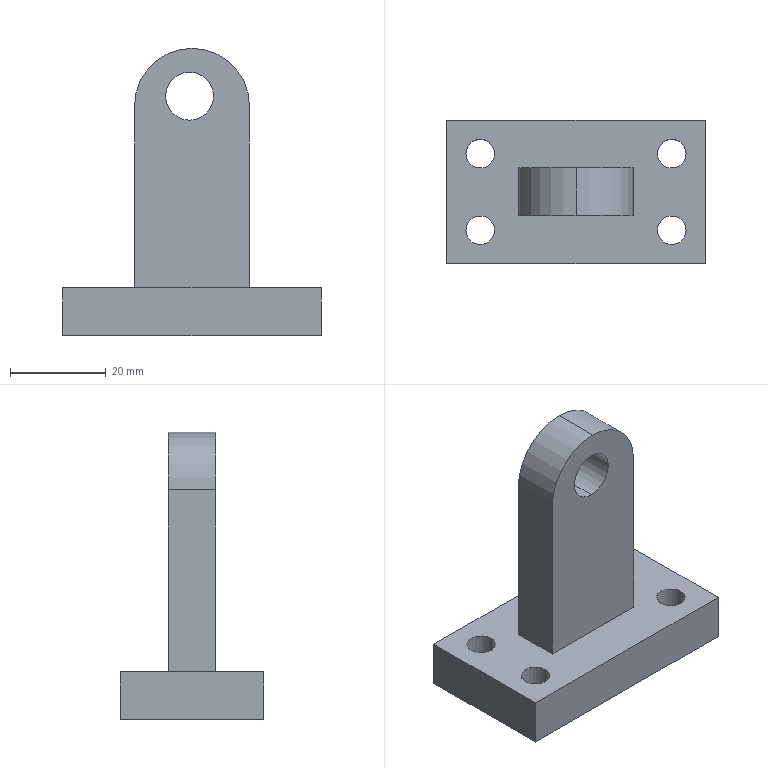Part | SolidWorks | features ICE 2, Extrusion 1, Fillet 1 | 1 solid | 22 faces | box 54 x 30 x 60 mm | volume 25666 mm3 | cylinder 12 | plane 10 | commonest cylinder face diameters 6 x8 10 x2 24 x2
STEP:
#1=CARTESIAN_POINT('',(26.5,20.,55.));
#2=VERTEX_POINT('',#1);
#3=CARTESIAN_POINT('',(26.5,20.,45.));
#4=VERTEX_POINT('',#3);
#5=CARTESIAN_POINT('',(26.5,20.,50.));
#6=DIRECTION('',(0.,-1.,0.));
#7=DIRECTION('',(0.,0.,-1.));
#8=AXIS2_PLACEMENT_3D('',#5,#6,#7);
#9=CIRCLE('',#8,5.);
#10=EDGE_CURVE('',#2,#4,#9,.T.);
#11=ORIENTED_EDGE('',*,*,#10,.F.);
#12=CARTESIAN_POINT('',(26.5,10.,55.));
#13=VERTEX_POINT('',#12);
#14=CARTESIAN_POINT('',(26.5,38.,55.));
#15=DIRECTION('',(0.,-1.,0.));
#16=VECTOR('',#15,1000.);
#17=LINE('',#14,#16);
#18=EDGE_CURVE('',#2,#13,#17,.T.);
#19=ORIENTED_EDGE('',*,*,#18,.T.);
#20=CARTESIAN_POINT('',(26.5,10.,45.));
#21=VERTEX_POINT('',#20);
#22=CARTESIAN_POINT('',(26.5,10.,50.));
#23=DIRECTION('',(0.,-1.,0.));
#24=DIRECTION('',(0.,0.,-1.));
#25=AXIS2_PLACEMENT_3D('',#22,#23,#24);
#26=CIRCLE('',#25,5.);
#27=EDGE_CURVE('',#13,#21,#26,.T.);
#28=ORIENTED_EDGE('',*,*,#27,.T.);
#29=CARTESIAN_POINT('',(26.5,38.,45.));
#30=DIRECTION('',(0.,-1.,0.));
#31=VECTOR('',#30,1000.);
#32=LINE('',#29,#31);
#33=EDGE_CURVE('',#4,#21,#32,.T.);
#34=ORIENTED_EDGE('',*,*,#33,.F.);
#35=EDGE_LOOP('',(#11,#19,#28,#34));
#36=FACE_OUTER_BOUND('',#35,.T.);
#37=CARTESIAN_POINT('',(26.5,38.,50.));
#38=DIRECTION('',(0.,-1.,0.));
#39=DIRECTION('',(0.,0.,-1.));
#40=AXIS2_PLACEMENT_3D('',#37,#38,#39);
#41=CYLINDRICAL_SURFACE('',#40,5.);
#42=ADVANCED_FACE('',(#36),#41,.F.);
#43=CARTESIAN_POINT('',(44.,7.,10.));
#44=VERTEX_POINT('',#43);
#45=CARTESIAN_POINT('',(50.,7.,10.));
#46=VERTEX_POINT('',#45);
#47=CARTESIAN_POINT('',(47.,7.,10.));
#48=DIRECTION('',(0.,0.,1.));
#49=DIRECTION('',(1.,0.,0.));
#50=AXIS2_PLACEMENT_3D('',#47,#48,#49);
#51=CIRCLE('',#50,3.);
#52=EDGE_CURVE('',#44,#46,#51,.T.);
#53=ORIENTED_EDGE('',*,*,#52,.T.);
#54=CARTESIAN_POINT('',(50.,7.,0.));
#55=VERTEX_POINT('',#54);
#56=CARTESIAN_POINT('',(50.,7.,10.));
#57=DIRECTION('',(0.,0.,-1.));
#58=VECTOR('',#57,1000.);
#59=LINE('',#56,#58);
#60=EDGE_CURVE('',#46,#55,#59,.T.);
#61=ORIENTED_EDGE('',*,*,#60,.T.);
#62=CARTESIAN_POINT('',(44.,7.,0.));
#63=VERTEX_POINT('',#62);
#64=CARTESIAN_POINT('',(47.,7.,0.));
#65=DIRECTION('',(0.,0.,1.));
#66=DIRECTION('',(1.,0.,0.));
#67=AXIS2_PLACEMENT_3D('',#64,#65,#66);
#68=CIRCLE('',#67,3.);
#69=EDGE_CURVE('',#63,#55,#68,.T.);
#70=ORIENTED_EDGE('',*,*,#69,.F.);
#71=CARTESIAN_POINT('',(44.,7.,10.));
#72=DIRECTION('',(0.,0.,-1.));
#73=VECTOR('',#72,1000.);
#74=LINE('',#71,#73);
#75=EDGE_CURVE('',#44,#63,#74,.T.);
#76=ORIENTED_EDGE('',*,*,#75,.F.);
#77=EDGE_LOOP('',(#53,#61,#70,#76));
#78=FACE_OUTER_BOUND('',#77,.T.);
#79=CARTESIAN_POINT('',(47.,7.,10.));
#80=DIRECTION('',(0.,0.,-1.));
#81=DIRECTION('',(-1.,0.,0.));
#82=AXIS2_PLACEMENT_3D('',#79,#80,#81);
#83=CYLINDRICAL_SURFACE('',#82,3.);
#84=ADVANCED_FACE('',(#78),#83,.F.);
#85=CARTESIAN_POINT('',(44.,23.,10.));
#86=VERTEX_POINT('',#85);
#87=CARTESIAN_POINT('',(50.,23.,10.));
#88=VERTEX_POINT('',#87);
#89=CARTESIAN_POINT('',(47.,23.,10.));
#90=DIRECTION('',(0.,0.,1.));
#91=DIRECTION('',(1.,0.,0.));
#92=AXIS2_PLACEMENT_3D('',#89,#90,#91);
#93=CIRCLE('',#92,3.);
#94=EDGE_CURVE('',#86,#88,#93,.T.);
#95=ORIENTED_EDGE('',*,*,#94,.T.);
#96=CARTESIAN_POINT('',(50.,23.,0.));
#97=VERTEX_POINT('',#96);
#98=CARTESIAN_POINT('',(50.,23.,10.));
#99=DIRECTION('',(0.,0.,-1.));
#100=VECTOR('',#99,1000.);
#101=LINE('',#98,#100);
#102=EDGE_CURVE('',#88,#97,#101,.T.);
#103=ORIENTED_EDGE('',*,*,#102,.T.);
#104=CARTESIAN_POINT('',(44.,23.,0.));
#105=VERTEX_POINT('',#104);
#106=CARTESIAN_POINT('',(47.,23.,0.));
#107=DIRECTION('',(0.,0.,1.));
#108=DIRECTION('',(1.,0.,0.));
#109=AXIS2_PLACEMENT_3D('',#106,#107,#108);
#110=CIRCLE('',#109,3.);
#111=EDGE_CURVE('',#105,#97,#110,.T.);
#112=ORIENTED_EDGE('',*,*,#111,.F.);
#113=CARTESIAN_POINT('',(44.,23.,10.));
#114=DIRECTION('',(0.,0.,-1.));
#115=VECTOR('',#114,1000.);
#116=LINE('',#113,#115);
#117=EDGE_CURVE('',#86,#105,#116,.T.);
#118=ORIENTED_EDGE('',*,*,#117,.F.);
#119=EDGE_LOOP('',(#95,#103,#112,#118));
#120=FACE_OUTER_BOUND('',#119,.T.);
#121=CARTESIAN_POINT('',(47.,23.,10.));
#122=DIRECTION('',(0.,0.,-1.));
#123=DIRECTION('',(-1.,0.,0.));
#124=AXIS2_PLACEMENT_3D('',#121,#122,#123);
#125=CYLINDRICAL_SURFACE('',#124,3.);
#126=ADVANCED_FACE('',(#120),#125,.F.);
#127=CARTESIAN_POINT('',(4.,7.,10.));
#128=VERTEX_POINT('',#127);
#129=CARTESIAN_POINT('',(10.,7.,10.));
#130=VERTEX_POINT('',#129);
#131=CARTESIAN_POINT('',(7.,7.,10.));
#132=DIRECTION('',(0.,0.,1.));
#133=DIRECTION('',(1.,0.,0.));
#134=AXIS2_PLACEMENT_3D('',#131,#132,#133);
#135=CIRCLE('',#134,3.);
#136=EDGE_CURVE('',#128,#130,#135,.T.);
#137=ORIENTED_EDGE('',*,*,#136,.T.);
#138=CARTESIAN_POINT('',(10.,7.,0.));
#139=VERTEX_POINT('',#138);
#140=CARTESIAN_POINT('',(10.,7.,10.));
#141=DIRECTION('',(0.,0.,-1.));
#142=VECTOR('',#141,1000.);
#143=LINE('',#140,#142);
#144=EDGE_CURVE('',#130,#139,#143,.T.);
#145=ORIENTED_EDGE('',*,*,#144,.T.);
#146=CARTESIAN_POINT('',(4.,7.,0.));
#147=VERTEX_POINT('',#146);
#148=CARTESIAN_POINT('',(7.,7.,0.));
#149=DIRECTION('',(0.,0.,1.));
#150=DIRECTION('',(1.,0.,0.));
#151=AXIS2_PLACEMENT_3D('',#148,#149,#150);
#152=CIRCLE('',#151,3.);
#153=EDGE_CURVE('',#147,#139,#152,.T.);
#154=ORIENTED_EDGE('',*,*,#153,.F.);
#155=CARTESIAN_POINT('',(4.,7.,10.));
#156=DIRECTION('',(0.,0.,-1.));
#157=VECTOR('',#156,1000.);
#158=LINE('',#155,#157);
#159=EDGE_CURVE('',#128,#147,#158,.T.);
#160=ORIENTED_EDGE('',*,*,#159,.F.);
#161=EDGE_LOOP('',(#137,#145,#154,#160));
#162=FACE_OUTER_BOUND('',#161,.T.);
#163=CARTESIAN_POINT('',(7.,7.,10.));
#164=DIRECTION('',(0.,0.,-1.));
#165=DIRECTION('',(-1.,0.,0.));
#166=AXIS2_PLACEMENT_3D('',#163,#164,#165);
#167=CYLINDRICAL_SURFACE('',#166,3.);
#168=ADVANCED_FACE('',(#162),#167,.F.);
#169=CARTESIAN_POINT('',(4.,23.,10.));
#170=VERTEX_POINT('',#169);
#171=CARTESIAN_POINT('',(10.,23.,10.));
#172=VERTEX_POINT('',#171);
#173=CARTESIAN_POINT('',(7.,23.,10.));
#174=DIRECTION('',(0.,0.,1.));
#175=DIRECTION('',(1.,0.,0.));
#176=AXIS2_PLACEMENT_3D('',#173,#174,#175);
#177=CIRCLE('',#176,3.);
#178=EDGE_CURVE('',#170,#172,#177,.T.);
#179=ORIENTED_EDGE('',*,*,#178,.T.);
#180=CARTESIAN_POINT('',(10.,23.,0.));
#181=VERTEX_POINT('',#180);
#182=CARTESIAN_POINT('',(10.,23.,10.));
#183=DIRECTION('',(0.,0.,-1.));
#184=VECTOR('',#183,1000.);
#185=LINE('',#182,#184);
#186=EDGE_CURVE('',#172,#181,#185,.T.);
#187=ORIENTED_EDGE('',*,*,#186,.T.);
#188=CARTESIAN_POINT('',(4.,23.,0.));
#189=VERTEX_POINT('',#188);
#190=CARTESIAN_POINT('',(7.,23.,0.));
#191=DIRECTION('',(0.,0.,1.));
#192=DIRECTION('',(1.,0.,0.));
#193=AXIS2_PLACEMENT_3D('',#190,#191,#192);
#194=CIRCLE('',#193,3.);
#195=EDGE_CURVE('',#189,#181,#194,.T.);
#196=ORIENTED_EDGE('',*,*,#195,.F.);
#197=CARTESIAN_POINT('',(4.,23.,10.));
#198=DIRECTION('',(0.,0.,-1.));
#199=VECTOR('',#198,1000.);
#200=LINE('',#197,#199);
#201=EDGE_CURVE('',#170,#189,#200,.T.);
#202=ORIENTED_EDGE('',*,*,#201,.F.);
#203=EDGE_LOOP('',(#179,#187,#196,#202));
#204=FACE_OUTER_BOUND('',#203,.T.);
#205=CARTESIAN_POINT('',(7.,23.,10.));
#206=DIRECTION('',(0.,0.,-1.));
#207=DIRECTION('',(-1.,0.,0.));
#208=AXIS2_PLACEMENT_3D('',#205,#206,#207);
#209=CYLINDRICAL_SURFACE('',#208,3.);
#210=ADVANCED_FACE('',(#204),#209,.F.);
#211=ORIENTED_EDGE('',*,*,#52,.F.);
#212=CARTESIAN_POINT('',(47.,7.,10.));
#213=DIRECTION('',(0.,0.,1.));
#214=DIRECTION('',(1.,0.,0.));
#215=AXIS2_PLACEMENT_3D('',#212,#213,#214);
#216=CIRCLE('',#215,3.);
#217=EDGE_CURVE('',#46,#44,#216,.T.);
#218=ORIENTED_EDGE('',*,*,#217,.F.);
#219=EDGE_LOOP('',(#211,#218));
#220=FACE_BOUND('',#219,.T.);
#221=ORIENTED_EDGE('',*,*,#94,.F.);
#222=CARTESIAN_POINT('',(47.,23.,10.));
#223=DIRECTION('',(0.,0.,1.));
#224=DIRECTION('',(1.,0.,0.));
#225=AXIS2_PLACEMENT_3D('',#222,#223,#224);
#226=CIRCLE('',#225,3.);
#227=EDGE_CURVE('',#88,#86,#226,.T.);
#228=ORIENTED_EDGE('',*,*,#227,.F.);
#229=EDGE_LOOP('',(#221,#228));
#230=FACE_BOUND('',#229,.T.);
#231=ORIENTED_EDGE('',*,*,#136,.F.);
#232=CARTESIAN_POINT('',(7.,7.,10.));
#233=DIRECTION('',(0.,0.,1.));
#234=DIRECTION('',(1.,0.,0.));
#235=AXIS2_PLACEMENT_3D('',#232,#233,#234);
#236=CIRCLE('',#235,3.);
#237=EDGE_CURVE('',#130,#128,#236,.T.);
#238=ORIENTED_EDGE('',*,*,#237,.F.);
#239=EDGE_LOOP('',(#231,#238));
#240=FACE_BOUND('',#239,.T.);
#241=ORIENTED_EDGE('',*,*,#178,.F.);
#242=CARTESIAN_POINT('',(7.,23.,10.));
#243=DIRECTION('',(0.,0.,1.));
#244=DIRECTION('',(1.,0.,0.));
#245=AXIS2_PLACEMENT_3D('',#242,#243,#244);
#246=CIRCLE('',#245,3.);
#247=EDGE_CURVE('',#172,#170,#246,.T.);
#248=ORIENTED_EDGE('',*,*,#247,.F.);
#249=EDGE_LOOP('',(#241,#248));
#250=FACE_BOUND('',#249,.T.);
#251=CARTESIAN_POINT('',(0.,30.,10.));
#252=VERTEX_POINT('',#251);
#253=CARTESIAN_POINT('',(0.,0.,10.));
#254=VERTEX_POINT('',#253);
#255=CARTESIAN_POINT('',(0.,0.,10.));
#256=DIRECTION('',(0.,-1.,0.));
#257=VECTOR('',#256,1000.);
#258=LINE('',#255,#257);
#259=EDGE_CURVE('',#252,#254,#258,.T.);
#260=ORIENTED_EDGE('',*,*,#259,.T.);
#261=CARTESIAN_POINT('',(54.,0.,10.));
#262=VERTEX_POINT('',#261);
#263=CARTESIAN_POINT('',(0.,0.,10.));
#264=DIRECTION('',(1.,0.,0.));
#265=VECTOR('',#264,1000.);
#266=LINE('',#263,#265);
#267=EDGE_CURVE('',#254,#262,#266,.T.);
#268=ORIENTED_EDGE('',*,*,#267,.T.);
#269=CARTESIAN_POINT('',(54.,30.,10.));
#270=VERTEX_POINT('',#269);
#271=CARTESIAN_POINT('',(54.,0.,10.));
#272=DIRECTION('',(0.,1.,0.));
#273=VECTOR('',#272,1000.);
#274=LINE('',#271,#273);
#275=EDGE_CURVE('',#262,#270,#274,.T.);
#276=ORIENTED_EDGE('',*,*,#275,.T.);
#277=CARTESIAN_POINT('',(0.,30.,10.));
#278=DIRECTION('',(-1.,0.,0.));
#279=VECTOR('',#278,1000.);
#280=LINE('',#277,#279);
#281=EDGE_CURVE('',#270,#252,#280,.T.);
#282=ORIENTED_EDGE('',*,*,#281,.T.);
#283=EDGE_LOOP('',(#260,#268,#276,#282));
#284=FACE_OUTER_BOUND('',#283,.T.);
#285=CARTESIAN_POINT('',(15.,20.,10.));
#286=VERTEX_POINT('',#285);
#287=CARTESIAN_POINT('',(15.,10.,10.));
#288=VERTEX_POINT('',#287);
#289=CARTESIAN_POINT('',(15.,20.,10.));
#290=DIRECTION('',(0.,-1.,0.));
#291=VECTOR('',#290,1000.);
#292=LINE('',#289,#291);
#293=EDGE_CURVE('',#286,#288,#292,.T.);
#294=ORIENTED_EDGE('',*,*,#293,.F.);
#295=CARTESIAN_POINT('',(39.,20.,10.));
#296=VERTEX_POINT('',#295);
#297=CARTESIAN_POINT('',(15.,20.,10.));
#298=DIRECTION('',(-1.,0.,0.));
#299=VECTOR('',#298,1000.);
#300=LINE('',#297,#299);
#301=EDGE_CURVE('',#296,#286,#300,.T.);
#302=ORIENTED_EDGE('',*,*,#301,.F.);
#303=CARTESIAN_POINT('',(39.,10.,10.));
#304=VERTEX_POINT('',#303);
#305=CARTESIAN_POINT('',(39.,20.,10.));
#306=DIRECTION('',(0.,1.,0.));
#307=VECTOR('',#306,1000.);
#308=LINE('',#305,#307);
#309=EDGE_CURVE('',#304,#296,#308,.T.);
#310=ORIENTED_EDGE('',*,*,#309,.F.);
#311=CARTESIAN_POINT('',(15.,10.,10.));
#312=DIRECTION('',(1.,0.,0.));
#313=VECTOR('',#312,1000.);
#314=LINE('',#311,#313);
#315=EDGE_CURVE('',#288,#304,#314,.T.);
#316=ORIENTED_EDGE('',*,*,#315,.F.);
#317=EDGE_LOOP('',(#294,#302,#310,#316));
#318=FACE_BOUND('',#317,.T.);
#319=CARTESIAN_POINT('',(0.,0.,10.));
#320=DIRECTION('',(0.,0.,-1.));
#321=DIRECTION('',(-1.,0.,0.));
#322=AXIS2_PLACEMENT_3D('',#319,#320,#321);
#323=PLANE('',#322);
#324=ADVANCED_FACE('',(#220,#230,#240,#250,#284,#318),#323,.F.);
#325=ORIENTED_EDGE('',*,*,#111,.T.);
#326=CARTESIAN_POINT('',(47.,23.,0.));
#327=DIRECTION('',(0.,0.,1.));
#328=DIRECTION('',(1.,0.,0.));
#329=AXIS2_PLACEMENT_3D('',#326,#327,#328);
#330=CIRCLE('',#329,3.);
#331=EDGE_CURVE('',#97,#105,#330,.T.);
#332=ORIENTED_EDGE('',*,*,#331,.T.);
#333=EDGE_LOOP('',(#325,#332));
#334=FACE_BOUND('',#333,.T.);
#335=ORIENTED_EDGE('',*,*,#195,.T.);
#336=CARTESIAN_POINT('',(7.,23.,0.));
#337=DIRECTION('',(0.,0.,1.));
#338=DIRECTION('',(1.,0.,0.));
#339=AXIS2_PLACEMENT_3D('',#336,#337,#338);
#340=CIRCLE('',#339,3.);
#341=EDGE_CURVE('',#181,#189,#340,.T.);
#342=ORIENTED_EDGE('',*,*,#341,.T.);
#343=EDGE_LOOP('',(#335,#342));
#344=FACE_BOUND('',#343,.T.);
#345=CARTESIAN_POINT('',(0.,30.,0.));
#346=VERTEX_POINT('',#345);
#347=CARTESIAN_POINT('',(0.,0.,0.));
#348=VERTEX_POINT('',#347);
#349=CARTESIAN_POINT('',(0.,0.,0.));
#350=DIRECTION('',(0.,-1.,0.));
#351=VECTOR('',#350,1000.);
#352=LINE('',#349,#351);
#353=EDGE_CURVE('',#346,#348,#352,.T.);
#354=ORIENTED_EDGE('',*,*,#353,.F.);
#355=CARTESIAN_POINT('',(54.,30.,0.));
#356=VERTEX_POINT('',#355);
#357=CARTESIAN_POINT('',(0.,30.,0.));
#358=DIRECTION('',(-1.,0.,0.));
#359=VECTOR('',#358,1000.);
#360=LINE('',#357,#359);
#361=EDGE_CURVE('',#356,#346,#360,.T.);
#362=ORIENTED_EDGE('',*,*,#361,.F.);
#363=CARTESIAN_POINT('',(54.,0.,0.));
#364=VERTEX_POINT('',#363);
#365=CARTESIAN_POINT('',(54.,0.,0.));
#366=DIRECTION('',(0.,1.,0.));
#367=VECTOR('',#366,1000.);
#368=LINE('',#365,#367);
#369=EDGE_CURVE('',#364,#356,#368,.T.);
#370=ORIENTED_EDGE('',*,*,#369,.F.);
#371=CARTESIAN_POINT('',(0.,0.,0.));
#372=DIRECTION('',(1.,0.,0.));
#373=VECTOR('',#372,1000.);
#374=LINE('',#371,#373);
#375=EDGE_CURVE('',#348,#364,#374,.T.);
#376=ORIENTED_EDGE('',*,*,#375,.F.);
#377=EDGE_LOOP('',(#354,#362,#370,#376));
#378=FACE_OUTER_BOUND('',#377,.T.);
#379=ORIENTED_EDGE('',*,*,#153,.T.);
#380=CARTESIAN_POINT('',(7.,7.,0.));
#381=DIRECTION('',(0.,0.,1.));
#382=DIRECTION('',(1.,0.,0.));
#383=AXIS2_PLACEMENT_3D('',#380,#381,#382);
#384=CIRCLE('',#383,3.);
#385=EDGE_CURVE('',#139,#147,#384,.T.);
#386=ORIENTED_EDGE('',*,*,#385,.T.);
#387=EDGE_LOOP('',(#379,#386));
#388=FACE_BOUND('',#387,.T.);
#389=ORIENTED_EDGE('',*,*,#69,.T.);
#390=CARTESIAN_POINT('',(47.,7.,0.));
#391=DIRECTION('',(0.,0.,1.));
#392=DIRECTION('',(1.,0.,0.));
#393=AXIS2_PLACEMENT_3D('',#390,#391,#392);
#394=CIRCLE('',#393,3.);
#395=EDGE_CURVE('',#55,#63,#394,.T.);
#396=ORIENTED_EDGE('',*,*,#395,.T.);
#397=EDGE_LOOP('',(#389,#396));
#398=FACE_BOUND('',#397,.T.);
#399=CARTESIAN_POINT('',(0.,0.,0.));
#400=DIRECTION('',(0.,0.,-1.));
#401=DIRECTION('',(-1.,0.,0.));
#402=AXIS2_PLACEMENT_3D('',#399,#400,#401);
#403=PLANE('',#402);
#404=ADVANCED_FACE('',(#334,#344,#378,#388,#398),#403,.T.);
#405=ORIENTED_EDGE('',*,*,#353,.T.);
#406=CARTESIAN_POINT('',(0.,0.,10.));
#407=DIRECTION('',(0.,0.,-1.));
#408=VECTOR('',#407,1000.);
#409=LINE('',#406,#408);
#410=EDGE_CURVE('',#254,#348,#409,.T.);
#411=ORIENTED_EDGE('',*,*,#410,.F.);
#412=ORIENTED_EDGE('',*,*,#259,.F.);
#413=CARTESIAN_POINT('',(0.,30.,10.));
#414=DIRECTION('',(0.,0.,-1.));
#415=VECTOR('',#414,1000.);
#416=LINE('',#413,#415);
#417=EDGE_CURVE('',#252,#346,#416,.T.);
#418=ORIENTED_EDGE('',*,*,#417,.T.);
#419=EDGE_LOOP('',(#405,#411,#412,#418));
#420=FACE_OUTER_BOUND('',#419,.T.);
#421=CARTESIAN_POINT('',(0.,0.,10.));
#422=DIRECTION('',(1.,0.,0.));
#423=DIRECTION('',(0.,0.,-1.));
#424=AXIS2_PLACEMENT_3D('',#421,#422,#423);
#425=PLANE('',#424);
#426=ADVANCED_FACE('',(#420),#425,.F.);
#427=ORIENTED_EDGE('',*,*,#375,.T.);
#428=CARTESIAN_POINT('',(54.,0.,10.));
#429=DIRECTION('',(0.,0.,-1.));
#430=VECTOR('',#429,1000.);
#431=LINE('',#428,#430);
#432=EDGE_CURVE('',#262,#364,#431,.T.);
#433=ORIENTED_EDGE('',*,*,#432,.F.);
#434=ORIENTED_EDGE('',*,*,#267,.F.);
#435=ORIENTED_EDGE('',*,*,#410,.T.);
#436=EDGE_LOOP('',(#427,#433,#434,#435));
#437=FACE_OUTER_BOUND('',#436,.T.);
#438=CARTESIAN_POINT('',(0.,0.,10.));
#439=DIRECTION('',(0.,1.,0.));
#440=DIRECTION('',(0.,0.,1.));
#441=AXIS2_PLACEMENT_3D('',#438,#439,#440);
#442=PLANE('',#441);
#443=ADVANCED_FACE('',(#437),#442,.F.);
#444=ORIENTED_EDGE('',*,*,#369,.T.);
#445=CARTESIAN_POINT('',(54.,30.,10.));
#446=DIRECTION('',(0.,0.,-1.));
#447=VECTOR('',#446,1000.);
#448=LINE('',#445,#447);
#449=EDGE_CURVE('',#270,#356,#448,.T.);
#450=ORIENTED_EDGE('',*,*,#449,.F.);
#451=ORIENTED_EDGE('',*,*,#275,.F.);
#452=ORIENTED_EDGE('',*,*,#432,.T.);
#453=EDGE_LOOP('',(#444,#450,#451,#452));
#454=FACE_OUTER_BOUND('',#453,.T.);
#455=CARTESIAN_POINT('',(54.,0.,10.));
#456=DIRECTION('',(-1.,0.,0.));
#457=DIRECTION('',(0.,0.,1.));
#458=AXIS2_PLACEMENT_3D('',#455,#456,#457);
#459=PLANE('',#458);
#460=ADVANCED_FACE('',(#454),#459,.F.);
#461=ORIENTED_EDGE('',*,*,#361,.T.);
#462=ORIENTED_EDGE('',*,*,#417,.F.);
#463=ORIENTED_EDGE('',*,*,#281,.F.);
#464=ORIENTED_EDGE('',*,*,#449,.T.);
#465=EDGE_LOOP('',(#461,#462,#463,#464));
#466=FACE_OUTER_BOUND('',#465,.T.);
#467=CARTESIAN_POINT('',(0.,30.,10.));
#468=DIRECTION('',(0.,-1.,0.));
#469=DIRECTION('',(0.,0.,-1.));
#470=AXIS2_PLACEMENT_3D('',#467,#468,#469);
#471=PLANE('',#470);
#472=ADVANCED_FACE('',(#466),#471,.F.);
#473=ORIENTED_EDGE('',*,*,#186,.F.);
#474=ORIENTED_EDGE('',*,*,#247,.T.);
#475=ORIENTED_EDGE('',*,*,#201,.T.);
#476=ORIENTED_EDGE('',*,*,#341,.F.);
#477=EDGE_LOOP('',(#473,#474,#475,#476));
#478=FACE_OUTER_BOUND('',#477,.T.);
#479=CARTESIAN_POINT('',(7.,23.,10.));
#480=DIRECTION('',(0.,0.,-1.));
#481=DIRECTION('',(-1.,0.,0.));
#482=AXIS2_PLACEMENT_3D('',#479,#480,#481);
#483=CYLINDRICAL_SURFACE('',#482,3.);
#484=ADVANCED_FACE('',(#478),#483,.F.);
#485=ORIENTED_EDGE('',*,*,#144,.F.);
#486=ORIENTED_EDGE('',*,*,#237,.T.);
#487=ORIENTED_EDGE('',*,*,#159,.T.);
#488=ORIENTED_EDGE('',*,*,#385,.F.);
#489=EDGE_LOOP('',(#485,#486,#487,#488));
#490=FACE_OUTER_BOUND('',#489,.T.);
#491=CARTESIAN_POINT('',(7.,7.,10.));
#492=DIRECTION('',(0.,0.,-1.));
#493=DIRECTION('',(-1.,0.,0.));
#494=AXIS2_PLACEMENT_3D('',#491,#492,#493);
#495=CYLINDRICAL_SURFACE('',#494,3.);
#496=ADVANCED_FACE('',(#490),#495,.F.);
#497=ORIENTED_EDGE('',*,*,#102,.F.);
#498=ORIENTED_EDGE('',*,*,#227,.T.);
#499=ORIENTED_EDGE('',*,*,#117,.T.);
#500=ORIENTED_EDGE('',*,*,#331,.F.);
#501=EDGE_LOOP('',(#497,#498,#499,#500));
#502=FACE_OUTER_BOUND('',#501,.T.);
#503=CARTESIAN_POINT('',(47.,23.,10.));
#504=DIRECTION('',(0.,0.,-1.));
#505=DIRECTION('',(-1.,0.,0.));
#506=AXIS2_PLACEMENT_3D('',#503,#504,#505);
#507=CYLINDRICAL_SURFACE('',#506,3.);
#508=ADVANCED_FACE('',(#502),#507,.F.);
#509=ORIENTED_EDGE('',*,*,#60,.F.);
#510=ORIENTED_EDGE('',*,*,#217,.T.);
#511=ORIENTED_EDGE('',*,*,#75,.T.);
#512=ORIENTED_EDGE('',*,*,#395,.F.);
#513=EDGE_LOOP('',(#509,#510,#511,#512));
#514=FACE_OUTER_BOUND('',#513,.T.);
#515=CARTESIAN_POINT('',(47.,7.,10.));
#516=DIRECTION('',(0.,0.,-1.));
#517=DIRECTION('',(-1.,0.,0.));
#518=AXIS2_PLACEMENT_3D('',#515,#516,#517);
#519=CYLINDRICAL_SURFACE('',#518,3.);
#520=ADVANCED_FACE('',(#514),#519,.F.);
#521=CARTESIAN_POINT('',(15.,10.,48.));
#522=VERTEX_POINT('',#521);
#523=CARTESIAN_POINT('',(15.,10.,60.));
#524=DIRECTION('',(0.,0.,-1.));
#525=VECTOR('',#524,1000.);
#526=LINE('',#523,#525);
#527=EDGE_CURVE('',#522,#288,#526,.T.);
#528=ORIENTED_EDGE('',*,*,#527,.F.);
#529=CARTESIAN_POINT('',(15.,20.,48.));
#530=VERTEX_POINT('',#529);
#531=CARTESIAN_POINT('',(15.,20.,48.));
#532=DIRECTION('',(0.,1.,0.));
#533=VECTOR('',#532,1000.);
#534=LINE('',#531,#533);
#535=EDGE_CURVE('',#522,#530,#534,.T.);
#536=ORIENTED_EDGE('',*,*,#535,.T.);
#537=CARTESIAN_POINT('',(15.,20.,60.));
#538=DIRECTION('',(0.,0.,-1.));
#539=VECTOR('',#538,1000.);
#540=LINE('',#537,#539);
#541=EDGE_CURVE('',#530,#286,#540,.T.);
#542=ORIENTED_EDGE('',*,*,#541,.T.);
#543=ORIENTED_EDGE('',*,*,#293,.T.);
#544=EDGE_LOOP('',(#528,#536,#542,#543));
#545=FACE_OUTER_BOUND('',#544,.T.);
#546=CARTESIAN_POINT('',(15.,20.,60.));
#547=DIRECTION('',(1.,0.,0.));
#548=DIRECTION('',(0.,1.,0.));
#549=AXIS2_PLACEMENT_3D('',#546,#547,#548);
#550=PLANE('',#549);
#551=ADVANCED_FACE('',(#545),#550,.F.);
#552=CARTESIAN_POINT('',(26.5,10.,50.));
#553=DIRECTION('',(0.,-1.,0.));
#554=DIRECTION('',(0.,0.,-1.));
#555=AXIS2_PLACEMENT_3D('',#552,#553,#554);
#556=CIRCLE('',#555,5.);
#557=EDGE_CURVE('',#21,#13,#556,.T.);
#558=ORIENTED_EDGE('',*,*,#557,.F.);
#559=ORIENTED_EDGE('',*,*,#27,.F.);
#560=EDGE_LOOP('',(#558,#559));
#561=FACE_BOUND('',#560,.T.);
#562=CARTESIAN_POINT('',(39.,10.,48.));
#563=VERTEX_POINT('',#562);
#564=CARTESIAN_POINT('',(39.,10.,60.));
#565=DIRECTION('',(0.,0.,-1.));
#566=VECTOR('',#565,1000.);
#567=LINE('',#564,#566);
#568=EDGE_CURVE('',#563,#304,#567,.T.);
#569=ORIENTED_EDGE('',*,*,#568,.F.);
#570=CARTESIAN_POINT('',(27.,10.,60.));
#571=VERTEX_POINT('',#570);
#572=CARTESIAN_POINT('',(27.,10.,48.));
#573=DIRECTION('',(0.,-1.,0.));
#574=DIRECTION('',(0.,0.,1.));
#575=AXIS2_PLACEMENT_3D('',#572,#573,#574);
#576=CIRCLE('',#575,12.);
#577=EDGE_CURVE('',#563,#571,#576,.T.);
#578=ORIENTED_EDGE('',*,*,#577,.T.);
#579=CARTESIAN_POINT('',(27.,10.,48.));
#580=DIRECTION('',(0.,-1.,0.));
#581=DIRECTION('',(0.,0.,1.));
#582=AXIS2_PLACEMENT_3D('',#579,#580,#581);
#583=CIRCLE('',#582,12.);
#584=EDGE_CURVE('',#571,#522,#583,.T.);
#585=ORIENTED_EDGE('',*,*,#584,.T.);
#586=ORIENTED_EDGE('',*,*,#527,.T.);
#587=ORIENTED_EDGE('',*,*,#315,.T.);
#588=EDGE_LOOP('',(#569,#578,#585,#586,#587));
#589=FACE_OUTER_BOUND('',#588,.T.);
#590=CARTESIAN_POINT('',(15.,10.,60.));
#591=DIRECTION('',(0.,1.,0.));
#592=DIRECTION('',(0.,0.,1.));
#593=AXIS2_PLACEMENT_3D('',#590,#591,#592);
#594=PLANE('',#593);
#595=ADVANCED_FACE('',(#561,#589),#594,.F.);
#596=CARTESIAN_POINT('',(39.,20.,48.));
#597=VERTEX_POINT('',#596);
#598=CARTESIAN_POINT('',(39.,20.,60.));
#599=DIRECTION('',(0.,0.,-1.));
#600=VECTOR('',#599,1000.);
#601=LINE('',#598,#600);
#602=EDGE_CURVE('',#597,#296,#601,.T.);
#603=ORIENTED_EDGE('',*,*,#602,.F.);
#604=CARTESIAN_POINT('',(39.,10.,48.));
#605=DIRECTION('',(0.,-1.,0.));
#606=VECTOR('',#605,1000.);
#607=LINE('',#604,#606);
#608=EDGE_CURVE('',#597,#563,#607,.T.);
#609=ORIENTED_EDGE('',*,*,#608,.T.);
#610=ORIENTED_EDGE('',*,*,#568,.T.);
#611=ORIENTED_EDGE('',*,*,#309,.T.);
#612=EDGE_LOOP('',(#603,#609,#610,#611));
#613=FACE_OUTER_BOUND('',#612,.T.);
#614=CARTESIAN_POINT('',(39.,20.,60.));
#615=DIRECTION('',(-1.,0.,0.));
#616=DIRECTION('',(0.,0.,1.));
#617=AXIS2_PLACEMENT_3D('',#614,#615,#616);
#618=PLANE('',#617);
#619=ADVANCED_FACE('',(#613),#618,.F.);
#620=CARTESIAN_POINT('',(26.5,20.,50.));
#621=DIRECTION('',(0.,-1.,0.));
#622=DIRECTION('',(0.,0.,-1.));
#623=AXIS2_PLACEMENT_3D('',#620,#621,#622);
#624=CIRCLE('',#623,5.);
#625=EDGE_CURVE('',#4,#2,#624,.T.);
#626=ORIENTED_EDGE('',*,*,#625,.T.);
#627=ORIENTED_EDGE('',*,*,#10,.T.);
#628=EDGE_LOOP('',(#626,#627));
#629=FACE_BOUND('',#628,.T.);
#630=CARTESIAN_POINT('',(27.,20.,60.));
#631=VERTEX_POINT('',#630);
#632=CARTESIAN_POINT('',(27.,20.,48.));
#633=DIRECTION('',(0.,1.,0.));
#634=DIRECTION('',(0.,0.,-1.));
#635=AXIS2_PLACEMENT_3D('',#632,#633,#634);
#636=CIRCLE('',#635,12.);
#637=EDGE_CURVE('',#530,#631,#636,.T.);
#638=ORIENTED_EDGE('',*,*,#637,.T.);
#639=CARTESIAN_POINT('',(27.,20.,48.));
#640=DIRECTION('',(0.,1.,0.));
#641=DIRECTION('',(0.,0.,-1.));
#642=AXIS2_PLACEMENT_3D('',#639,#640,#641);
#643=CIRCLE('',#642,12.);
#644=EDGE_CURVE('',#631,#597,#643,.T.);
#645=ORIENTED_EDGE('',*,*,#644,.T.);
#646=ORIENTED_EDGE('',*,*,#602,.T.);
#647=ORIENTED_EDGE('',*,*,#301,.T.);
#648=ORIENTED_EDGE('',*,*,#541,.F.);
#649=EDGE_LOOP('',(#638,#645,#646,#647,#648));
#650=FACE_OUTER_BOUND('',#649,.T.);
#651=CARTESIAN_POINT('',(15.,20.,60.));
#652=DIRECTION('',(0.,-1.,0.));
#653=DIRECTION('',(0.,0.,-1.));
#654=AXIS2_PLACEMENT_3D('',#651,#652,#653);
#655=PLANE('',#654);
#656=ADVANCED_FACE('',(#629,#650),#655,.F.);
#657=ORIENTED_EDGE('',*,*,#18,.F.);
#658=ORIENTED_EDGE('',*,*,#625,.F.);
#659=ORIENTED_EDGE('',*,*,#33,.T.);
#660=ORIENTED_EDGE('',*,*,#557,.T.);
#661=EDGE_LOOP('',(#657,#658,#659,#660));
#662=FACE_OUTER_BOUND('',#661,.T.);
#663=CARTESIAN_POINT('',(26.5,38.,50.));
#664=DIRECTION('',(0.,-1.,0.));
#665=DIRECTION('',(0.,0.,-1.));
#666=AXIS2_PLACEMENT_3D('',#663,#664,#665);
#667=CYLINDRICAL_SURFACE('',#666,5.);
#668=ADVANCED_FACE('',(#662),#667,.F.);
#669=ORIENTED_EDGE('',*,*,#535,.F.);
#670=ORIENTED_EDGE('',*,*,#584,.F.);
#671=CARTESIAN_POINT('',(27.,10.,60.));
#672=DIRECTION('',(0.,-1.,0.));
#673=VECTOR('',#672,1000.);
#674=LINE('',#671,#673);
#675=EDGE_CURVE('',#631,#571,#674,.T.);
#676=ORIENTED_EDGE('',*,*,#675,.F.);
#677=ORIENTED_EDGE('',*,*,#637,.F.);
#678=EDGE_LOOP('',(#669,#670,#676,#677));
#679=FACE_OUTER_BOUND('',#678,.T.);
#680=CARTESIAN_POINT('',(27.,0.,48.));
#681=DIRECTION('',(0.,1.,0.));
#682=DIRECTION('',(-1.,0.,0.));
#683=AXIS2_PLACEMENT_3D('',#680,#681,#682);
#684=CYLINDRICAL_SURFACE('',#683,12.);
#685=ADVANCED_FACE('',(#679),#684,.T.);
#686=ORIENTED_EDGE('',*,*,#577,.F.);
#687=ORIENTED_EDGE('',*,*,#608,.F.);
#688=ORIENTED_EDGE('',*,*,#644,.F.);
#689=ORIENTED_EDGE('',*,*,#675,.T.);
#690=EDGE_LOOP('',(#686,#687,#688,#689));
#691=FACE_OUTER_BOUND('',#690,.T.);
#692=CARTESIAN_POINT('',(27.,0.,48.));
#693=DIRECTION('',(0.,-1.,0.));
#694=DIRECTION('',(0.,0.,-1.));
#695=AXIS2_PLACEMENT_3D('',#692,#693,#694);
#696=CYLINDRICAL_SURFACE('',#695,12.);
#697=ADVANCED_FACE('',(#691),#696,.T.);
#698=CLOSED_SHELL('',(#42,#84,#126,#168,#210,#324,#404,#426,#443,#460,#472,#484,#496,#508,#520,#551,#595,#619,#656,#668,#685,#697));
#699=MANIFOLD_SOLID_BREP('',#698);
#700=CARTESIAN_POINT('',(0.,0.,0.));
#701=DIRECTION('',(0.,0.,1.));
#702=DIRECTION('',(1.,0.,0.));
#703=AXIS2_PLACEMENT_3D('',#700,#701,#702);
#704=(LENGTH_UNIT()NAMED_UNIT(*)SI_UNIT(.MILLI.,.METRE.));
#705=UNCERTAINTY_MEASURE_WITH_UNIT(LENGTH_MEASURE(0.00001),#704,'','');
#706=(NAMED_UNIT(*)PLANE_ANGLE_UNIT()SI_UNIT($,.RADIAN.));
#707=(NAMED_UNIT(*)SI_UNIT($,.STERADIAN.)SOLID_ANGLE_UNIT());
#708=(GEOMETRIC_REPRESENTATION_CONTEXT(3)GLOBAL_UNCERTAINTY_ASSIGNED_CONTEXT((#705))GLOBAL_UNIT_ASSIGNED_CONTEXT((#704,#706,#707))REPRESENTATION_CONTEXT('',''));
#709=ADVANCED_BREP_SHAPE_REPRESENTATION('',(#699,#703),#708);